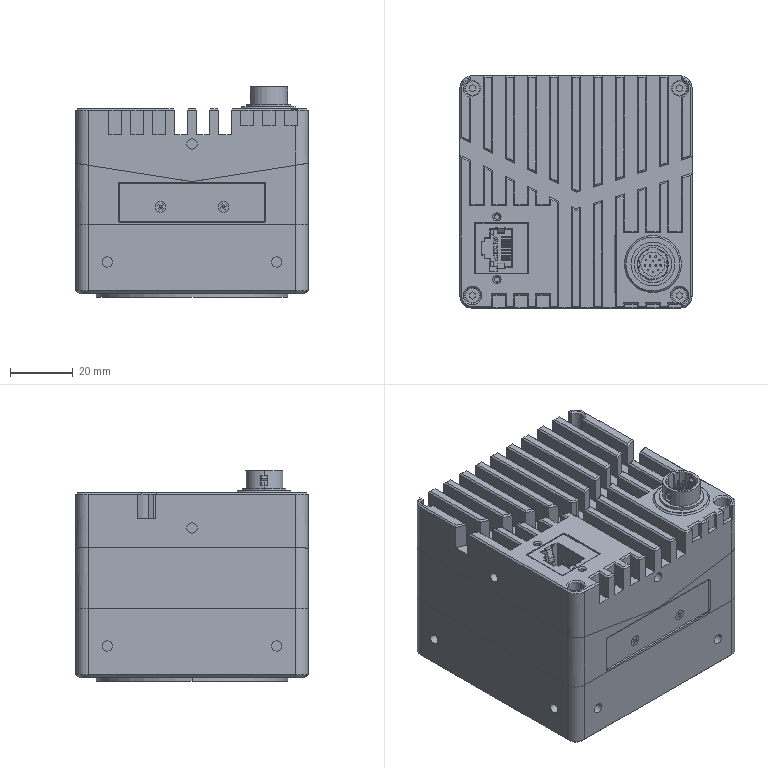Part | SolidWorks | features BaseBody 24 | 24 solids | 1825 faces | box 74 x 74 x 66.99 mm | volume 341850 mm3 | plane 1174 | cylinder 567 | cone 52 | spline 28 | torus 4 | commonest cylinder face diameters 2 x83 0.6 x56 0.5 x36 0.4 x32 2.5 x32 3.3 x32